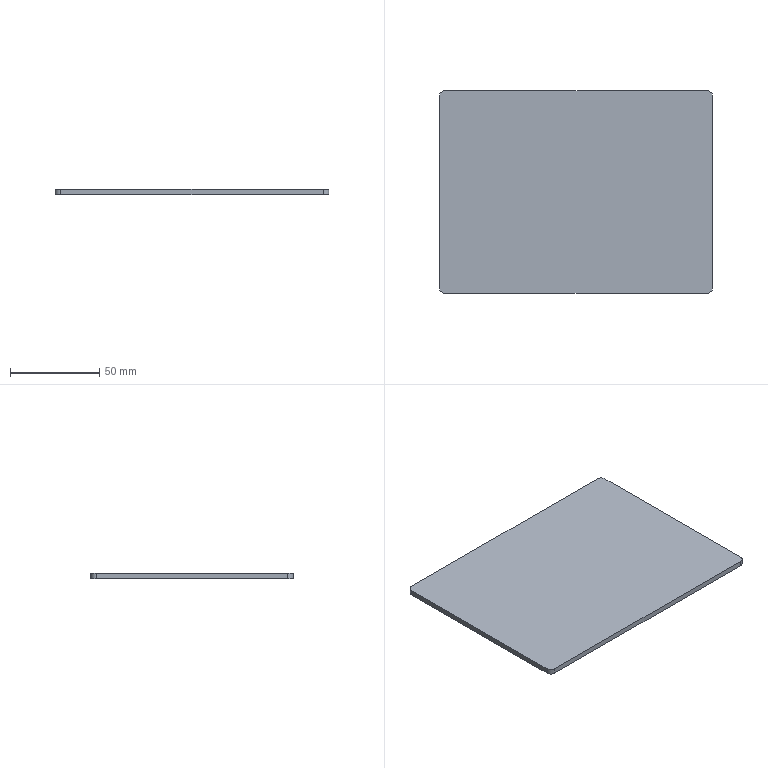Part | SolidWorks | features Extrusion 1, Fillet 1 | 1 solid | 10 faces | box 153.5 x 113.5 x 3 mm | volume 52244 mm3 | plane 6 | cylinder 4 | commonest cylinder face diameters 6 x4
STEP:
#1=CARTESIAN_POINT('',(32.634,47.448,0.));
#2=VERTEX_POINT('',#1);
#3=CARTESIAN_POINT('',(32.634,-60.052,0.));
#4=VERTEX_POINT('',#3);
#5=CARTESIAN_POINT('',(32.634,50.448,0.));
#6=DIRECTION('',(0.,-1.,0.));
#7=VECTOR('',#6,1000.);
#8=LINE('',#5,#7);
#9=EDGE_CURVE('',#2,#4,#8,.T.);
#10=ORIENTED_EDGE('',*,*,#9,.T.);
#11=CARTESIAN_POINT('',(32.634,-60.052,3.));
#12=VERTEX_POINT('',#11);
#13=CARTESIAN_POINT('',(32.634,-60.052,3.));
#14=DIRECTION('',(0.,0.,1.));
#15=VECTOR('',#14,1000.);
#16=LINE('',#13,#15);
#17=EDGE_CURVE('',#4,#12,#16,.T.);
#18=ORIENTED_EDGE('',*,*,#17,.T.);
#19=CARTESIAN_POINT('',(32.634,47.448,3.));
#20=VERTEX_POINT('',#19);
#21=CARTESIAN_POINT('',(32.634,50.448,3.));
#22=DIRECTION('',(0.,-1.,0.));
#23=VECTOR('',#22,1000.);
#24=LINE('',#21,#23);
#25=EDGE_CURVE('',#20,#12,#24,.T.);
#26=ORIENTED_EDGE('',*,*,#25,.F.);
#27=CARTESIAN_POINT('',(32.634,47.448,3.));
#28=DIRECTION('',(0.,0.,-1.));
#29=VECTOR('',#28,1000.);
#30=LINE('',#27,#29);
#31=EDGE_CURVE('',#20,#2,#30,.T.);
#32=ORIENTED_EDGE('',*,*,#31,.T.);
#33=EDGE_LOOP('',(#10,#18,#26,#32));
#34=FACE_OUTER_BOUND('',#33,.T.);
#35=CARTESIAN_POINT('',(32.634,50.448,3.));
#36=DIRECTION('',(1.,0.,0.));
#37=DIRECTION('',(0.,1.,0.));
#38=AXIS2_PLACEMENT_3D('',#35,#36,#37);
#39=PLANE('',#38);
#40=ADVANCED_FACE('',(#34),#39,.F.);
#41=CARTESIAN_POINT('',(35.634,-63.052,3.));
#42=VERTEX_POINT('',#41);
#43=CARTESIAN_POINT('',(183.134,-63.052,3.));
#44=VERTEX_POINT('',#43);
#45=CARTESIAN_POINT('',(32.634,-63.052,3.));
#46=DIRECTION('',(1.,0.,0.));
#47=VECTOR('',#46,1000.);
#48=LINE('',#45,#47);
#49=EDGE_CURVE('',#42,#44,#48,.T.);
#50=ORIENTED_EDGE('',*,*,#49,.F.);
#51=CARTESIAN_POINT('',(35.634,-63.052,0.));
#52=VERTEX_POINT('',#51);
#53=CARTESIAN_POINT('',(35.634,-63.052,3.));
#54=DIRECTION('',(0.,0.,-1.));
#55=VECTOR('',#54,1000.);
#56=LINE('',#53,#55);
#57=EDGE_CURVE('',#42,#52,#56,.T.);
#58=ORIENTED_EDGE('',*,*,#57,.T.);
#59=CARTESIAN_POINT('',(183.134,-63.052,0.));
#60=VERTEX_POINT('',#59);
#61=CARTESIAN_POINT('',(32.634,-63.052,0.));
#62=DIRECTION('',(1.,0.,0.));
#63=VECTOR('',#62,1000.);
#64=LINE('',#61,#63);
#65=EDGE_CURVE('',#52,#60,#64,.T.);
#66=ORIENTED_EDGE('',*,*,#65,.T.);
#67=CARTESIAN_POINT('',(183.134,-63.052,3.));
#68=DIRECTION('',(0.,0.,1.));
#69=VECTOR('',#68,1000.);
#70=LINE('',#67,#69);
#71=EDGE_CURVE('',#60,#44,#70,.T.);
#72=ORIENTED_EDGE('',*,*,#71,.T.);
#73=EDGE_LOOP('',(#50,#58,#66,#72));
#74=FACE_OUTER_BOUND('',#73,.T.);
#75=CARTESIAN_POINT('',(32.634,-63.052,3.));
#76=DIRECTION('',(0.,1.,0.));
#77=DIRECTION('',(0.,0.,1.));
#78=AXIS2_PLACEMENT_3D('',#75,#76,#77);
#79=PLANE('',#78);
#80=ADVANCED_FACE('',(#74),#79,.F.);
#81=CARTESIAN_POINT('',(186.134,-60.052,3.));
#82=VERTEX_POINT('',#81);
#83=CARTESIAN_POINT('',(186.134,47.448,3.));
#84=VERTEX_POINT('',#83);
#85=CARTESIAN_POINT('',(186.134,50.448,3.));
#86=DIRECTION('',(0.,1.,0.));
#87=VECTOR('',#86,1000.);
#88=LINE('',#85,#87);
#89=EDGE_CURVE('',#82,#84,#88,.T.);
#90=ORIENTED_EDGE('',*,*,#89,.F.);
#91=CARTESIAN_POINT('',(186.134,-60.052,0.));
#92=VERTEX_POINT('',#91);
#93=CARTESIAN_POINT('',(186.134,-60.052,3.));
#94=DIRECTION('',(0.,0.,-1.));
#95=VECTOR('',#94,1000.);
#96=LINE('',#93,#95);
#97=EDGE_CURVE('',#82,#92,#96,.T.);
#98=ORIENTED_EDGE('',*,*,#97,.T.);
#99=CARTESIAN_POINT('',(186.134,47.448,0.));
#100=VERTEX_POINT('',#99);
#101=CARTESIAN_POINT('',(186.134,50.448,0.));
#102=DIRECTION('',(0.,1.,0.));
#103=VECTOR('',#102,1000.);
#104=LINE('',#101,#103);
#105=EDGE_CURVE('',#92,#100,#104,.T.);
#106=ORIENTED_EDGE('',*,*,#105,.T.);
#107=CARTESIAN_POINT('',(186.134,47.448,3.));
#108=DIRECTION('',(0.,0.,1.));
#109=VECTOR('',#108,1000.);
#110=LINE('',#107,#109);
#111=EDGE_CURVE('',#100,#84,#110,.T.);
#112=ORIENTED_EDGE('',*,*,#111,.T.);
#113=EDGE_LOOP('',(#90,#98,#106,#112));
#114=FACE_OUTER_BOUND('',#113,.T.);
#115=CARTESIAN_POINT('',(186.134,50.448,3.));
#116=DIRECTION('',(-1.,0.,0.));
#117=DIRECTION('',(0.,-1.,0.));
#118=AXIS2_PLACEMENT_3D('',#115,#116,#117);
#119=PLANE('',#118);
#120=ADVANCED_FACE('',(#114),#119,.F.);
#121=CARTESIAN_POINT('',(183.134,50.448,3.));
#122=VERTEX_POINT('',#121);
#123=CARTESIAN_POINT('',(35.634,50.448,3.));
#124=VERTEX_POINT('',#123);
#125=CARTESIAN_POINT('',(32.634,50.448,3.));
#126=DIRECTION('',(-1.,0.,0.));
#127=VECTOR('',#126,1000.);
#128=LINE('',#125,#127);
#129=EDGE_CURVE('',#122,#124,#128,.T.);
#130=ORIENTED_EDGE('',*,*,#129,.F.);
#131=CARTESIAN_POINT('',(183.134,50.448,0.));
#132=VERTEX_POINT('',#131);
#133=CARTESIAN_POINT('',(183.134,50.448,3.));
#134=DIRECTION('',(0.,0.,-1.));
#135=VECTOR('',#134,1000.);
#136=LINE('',#133,#135);
#137=EDGE_CURVE('',#122,#132,#136,.T.);
#138=ORIENTED_EDGE('',*,*,#137,.T.);
#139=CARTESIAN_POINT('',(35.634,50.448,0.));
#140=VERTEX_POINT('',#139);
#141=CARTESIAN_POINT('',(32.634,50.448,0.));
#142=DIRECTION('',(-1.,0.,0.));
#143=VECTOR('',#142,1000.);
#144=LINE('',#141,#143);
#145=EDGE_CURVE('',#132,#140,#144,.T.);
#146=ORIENTED_EDGE('',*,*,#145,.T.);
#147=CARTESIAN_POINT('',(35.634,50.448,3.));
#148=DIRECTION('',(0.,0.,1.));
#149=VECTOR('',#148,1000.);
#150=LINE('',#147,#149);
#151=EDGE_CURVE('',#140,#124,#150,.T.);
#152=ORIENTED_EDGE('',*,*,#151,.T.);
#153=EDGE_LOOP('',(#130,#138,#146,#152));
#154=FACE_OUTER_BOUND('',#153,.T.);
#155=CARTESIAN_POINT('',(32.634,50.448,3.));
#156=DIRECTION('',(0.,-1.,0.));
#157=DIRECTION('',(0.,0.,-1.));
#158=AXIS2_PLACEMENT_3D('',#155,#156,#157);
#159=PLANE('',#158);
#160=ADVANCED_FACE('',(#154),#159,.F.);
#161=ORIENTED_EDGE('',*,*,#25,.T.);
#162=CARTESIAN_POINT('',(35.634,-60.052,3.));
#163=DIRECTION('',(0.,0.,1.));
#164=DIRECTION('',(1.,0.,0.));
#165=AXIS2_PLACEMENT_3D('',#162,#163,#164);
#166=CIRCLE('',#165,3.);
#167=EDGE_CURVE('',#12,#42,#166,.T.);
#168=ORIENTED_EDGE('',*,*,#167,.T.);
#169=ORIENTED_EDGE('',*,*,#49,.T.);
#170=CARTESIAN_POINT('',(183.134,-60.052,3.));
#171=DIRECTION('',(0.,0.,1.));
#172=DIRECTION('',(1.,0.,0.));
#173=AXIS2_PLACEMENT_3D('',#170,#171,#172);
#174=CIRCLE('',#173,3.);
#175=EDGE_CURVE('',#44,#82,#174,.T.);
#176=ORIENTED_EDGE('',*,*,#175,.T.);
#177=ORIENTED_EDGE('',*,*,#89,.T.);
#178=CARTESIAN_POINT('',(183.134,47.448,3.));
#179=DIRECTION('',(0.,0.,1.));
#180=DIRECTION('',(1.,0.,0.));
#181=AXIS2_PLACEMENT_3D('',#178,#179,#180);
#182=CIRCLE('',#181,3.);
#183=EDGE_CURVE('',#84,#122,#182,.T.);
#184=ORIENTED_EDGE('',*,*,#183,.T.);
#185=ORIENTED_EDGE('',*,*,#129,.T.);
#186=CARTESIAN_POINT('',(35.634,47.448,3.));
#187=DIRECTION('',(0.,0.,1.));
#188=DIRECTION('',(1.,0.,0.));
#189=AXIS2_PLACEMENT_3D('',#186,#187,#188);
#190=CIRCLE('',#189,3.);
#191=EDGE_CURVE('',#124,#20,#190,.T.);
#192=ORIENTED_EDGE('',*,*,#191,.T.);
#193=EDGE_LOOP('',(#161,#168,#169,#176,#177,#184,#185,#192));
#194=FACE_OUTER_BOUND('',#193,.T.);
#195=CARTESIAN_POINT('',(0.,0.,3.));
#196=DIRECTION('',(0.,0.,1.));
#197=DIRECTION('',(1.,0.,0.));
#198=AXIS2_PLACEMENT_3D('',#195,#196,#197);
#199=PLANE('',#198);
#200=ADVANCED_FACE('',(#194),#199,.T.);
#201=ORIENTED_EDGE('',*,*,#65,.F.);
#202=CARTESIAN_POINT('',(35.634,-60.052,0.));
#203=DIRECTION('',(0.,0.,-1.));
#204=DIRECTION('',(1.,0.,0.));
#205=AXIS2_PLACEMENT_3D('',#202,#203,#204);
#206=CIRCLE('',#205,3.);
#207=EDGE_CURVE('',#52,#4,#206,.T.);
#208=ORIENTED_EDGE('',*,*,#207,.T.);
#209=ORIENTED_EDGE('',*,*,#9,.F.);
#210=CARTESIAN_POINT('',(35.634,47.448,0.));
#211=DIRECTION('',(0.,0.,-1.));
#212=DIRECTION('',(1.,0.,0.));
#213=AXIS2_PLACEMENT_3D('',#210,#211,#212);
#214=CIRCLE('',#213,3.);
#215=EDGE_CURVE('',#2,#140,#214,.T.);
#216=ORIENTED_EDGE('',*,*,#215,.T.);
#217=ORIENTED_EDGE('',*,*,#145,.F.);
#218=CARTESIAN_POINT('',(183.134,47.448,0.));
#219=DIRECTION('',(0.,0.,-1.));
#220=DIRECTION('',(1.,0.,0.));
#221=AXIS2_PLACEMENT_3D('',#218,#219,#220);
#222=CIRCLE('',#221,3.);
#223=EDGE_CURVE('',#132,#100,#222,.T.);
#224=ORIENTED_EDGE('',*,*,#223,.T.);
#225=ORIENTED_EDGE('',*,*,#105,.F.);
#226=CARTESIAN_POINT('',(183.134,-60.052,0.));
#227=DIRECTION('',(0.,0.,-1.));
#228=DIRECTION('',(1.,0.,0.));
#229=AXIS2_PLACEMENT_3D('',#226,#227,#228);
#230=CIRCLE('',#229,3.);
#231=EDGE_CURVE('',#92,#60,#230,.T.);
#232=ORIENTED_EDGE('',*,*,#231,.T.);
#233=EDGE_LOOP('',(#201,#208,#209,#216,#217,#224,#225,#232));
#234=FACE_OUTER_BOUND('',#233,.T.);
#235=CARTESIAN_POINT('',(0.,0.,0.));
#236=DIRECTION('',(0.,0.,1.));
#237=DIRECTION('',(1.,0.,0.));
#238=AXIS2_PLACEMENT_3D('',#235,#236,#237);
#239=PLANE('',#238);
#240=ADVANCED_FACE('',(#234),#239,.F.);
#241=ORIENTED_EDGE('',*,*,#167,.F.);
#242=ORIENTED_EDGE('',*,*,#17,.F.);
#243=ORIENTED_EDGE('',*,*,#207,.F.);
#244=ORIENTED_EDGE('',*,*,#57,.F.);
#245=EDGE_LOOP('',(#241,#242,#243,#244));
#246=FACE_OUTER_BOUND('',#245,.T.);
#247=CARTESIAN_POINT('',(35.634,-60.052,3.));
#248=DIRECTION('',(0.,0.,-1.));
#249=DIRECTION('',(-1.,0.,0.));
#250=AXIS2_PLACEMENT_3D('',#247,#248,#249);
#251=CYLINDRICAL_SURFACE('',#250,3.);
#252=ADVANCED_FACE('',(#246),#251,.T.);
#253=ORIENTED_EDGE('',*,*,#175,.F.);
#254=ORIENTED_EDGE('',*,*,#71,.F.);
#255=ORIENTED_EDGE('',*,*,#231,.F.);
#256=ORIENTED_EDGE('',*,*,#97,.F.);
#257=EDGE_LOOP('',(#253,#254,#255,#256));
#258=FACE_OUTER_BOUND('',#257,.T.);
#259=CARTESIAN_POINT('',(183.134,-60.052,3.));
#260=DIRECTION('',(0.,0.,-1.));
#261=DIRECTION('',(-1.,0.,0.));
#262=AXIS2_PLACEMENT_3D('',#259,#260,#261);
#263=CYLINDRICAL_SURFACE('',#262,3.);
#264=ADVANCED_FACE('',(#258),#263,.T.);
#265=ORIENTED_EDGE('',*,*,#183,.F.);
#266=ORIENTED_EDGE('',*,*,#111,.F.);
#267=ORIENTED_EDGE('',*,*,#223,.F.);
#268=ORIENTED_EDGE('',*,*,#137,.F.);
#269=EDGE_LOOP('',(#265,#266,#267,#268));
#270=FACE_OUTER_BOUND('',#269,.T.);
#271=CARTESIAN_POINT('',(183.134,47.448,3.));
#272=DIRECTION('',(0.,0.,-1.));
#273=DIRECTION('',(-1.,0.,0.));
#274=AXIS2_PLACEMENT_3D('',#271,#272,#273);
#275=CYLINDRICAL_SURFACE('',#274,3.);
#276=ADVANCED_FACE('',(#270),#275,.T.);
#277=ORIENTED_EDGE('',*,*,#191,.F.);
#278=ORIENTED_EDGE('',*,*,#151,.F.);
#279=ORIENTED_EDGE('',*,*,#215,.F.);
#280=ORIENTED_EDGE('',*,*,#31,.F.);
#281=EDGE_LOOP('',(#277,#278,#279,#280));
#282=FACE_OUTER_BOUND('',#281,.T.);
#283=CARTESIAN_POINT('',(35.634,47.448,3.));
#284=DIRECTION('',(0.,0.,-1.));
#285=DIRECTION('',(-1.,0.,0.));
#286=AXIS2_PLACEMENT_3D('',#283,#284,#285);
#287=CYLINDRICAL_SURFACE('',#286,3.);
#288=ADVANCED_FACE('',(#282),#287,.T.);
#289=CLOSED_SHELL('',(#40,#80,#120,#160,#200,#240,#252,#264,#276,#288));
#290=MANIFOLD_SOLID_BREP('',#289);
#291=CARTESIAN_POINT('',(0.,0.,0.));
#292=DIRECTION('',(0.,0.,1.));
#293=DIRECTION('',(1.,0.,0.));
#294=AXIS2_PLACEMENT_3D('',#291,#292,#293);
#295=(LENGTH_UNIT()NAMED_UNIT(*)SI_UNIT(.MILLI.,.METRE.));
#296=UNCERTAINTY_MEASURE_WITH_UNIT(LENGTH_MEASURE(0.00001),#295,'','');
#297=(NAMED_UNIT(*)PLANE_ANGLE_UNIT()SI_UNIT($,.RADIAN.));
#298=(NAMED_UNIT(*)SI_UNIT($,.STERADIAN.)SOLID_ANGLE_UNIT());
#299=(GEOMETRIC_REPRESENTATION_CONTEXT(3)GLOBAL_UNCERTAINTY_ASSIGNED_CONTEXT((#296))GLOBAL_UNIT_ASSIGNED_CONTEXT((#295,#297,#298))REPRESENTATION_CONTEXT('',''));
#300=ADVANCED_BREP_SHAPE_REPRESENTATION('',(#290,#294),#299);